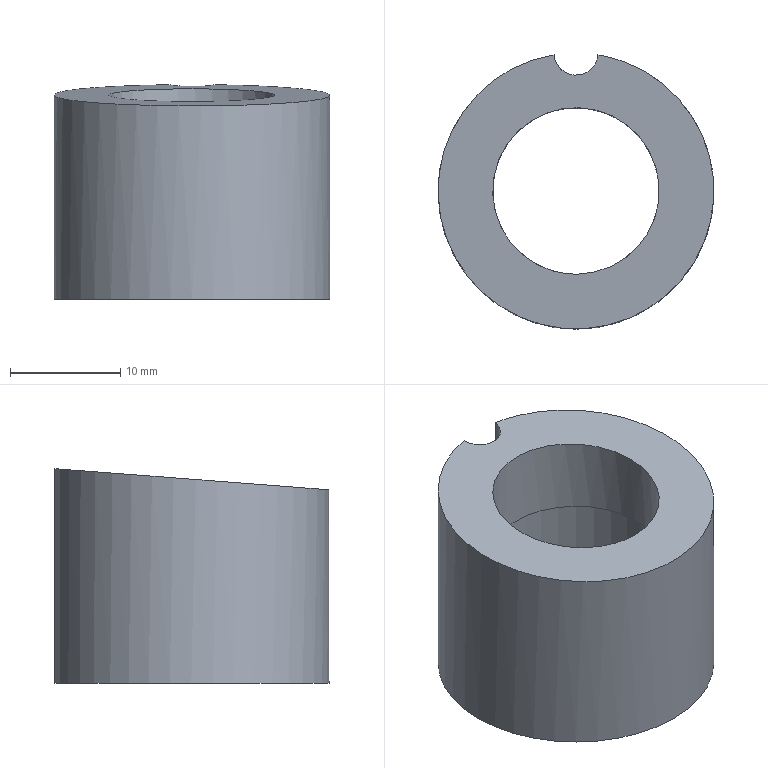Part | NX | features EKSD 25-20-15.10 2 | 1 solid | 7 faces | box 25 x 24.84 x 19.446 mm | volume 5201 mm3 | cylinder 4 | plane 3 | commonest cylinder face diameters 4 x1 15.1 x1 16.6 x1 25 x1
STEP:
#1=CARTESIAN_POINT('',(323.266,-25.835,-35.5));
#2=VERTEX_POINT('',#1);
#3=CARTESIAN_POINT('',(327.253,-25.835,-35.5));
#4=VERTEX_POINT('',#3);
#5=CARTESIAN_POINT('',(325.26,-25.675,-35.5));
#6=DIRECTION('',(0.,0.,1.));
#7=DIRECTION('',(1.,0.,0.));
#8=AXIS2_PLACEMENT_3D('',#5,#6,#7);
#9=CIRCLE('',#8,2.);
#10=EDGE_CURVE('',#2,#4,#9,.T.);
#11=ORIENTED_EDGE('',*,*,#10,.T.);
#12=CARTESIAN_POINT('',(325.26,-38.175,-35.5));
#13=DIRECTION('',(0.,0.,1.));
#14=DIRECTION('',(1.,0.,0.));
#15=AXIS2_PLACEMENT_3D('',#12,#13,#14);
#16=CIRCLE('',#15,12.5);
#17=EDGE_CURVE('',#2,#4,#16,.T.);
#18=ORIENTED_EDGE('',*,*,#17,.F.);
#19=EDGE_LOOP('',(#11,#18));
#20=FACE_BOUND('',#19,.T.);
#21=CARTESIAN_POINT('',(316.96,-38.175,-35.5));
#22=VERTEX_POINT('',#21);
#23=CARTESIAN_POINT('',(325.26,-38.175,-35.5));
#24=DIRECTION('',(0.,0.,-1.));
#25=DIRECTION('',(-1.,0.,0.));
#26=AXIS2_PLACEMENT_3D('',#23,#24,#25);
#27=CIRCLE('',#26,8.3);
#28=EDGE_CURVE('',#22,#22,#27,.T.);
#29=ORIENTED_EDGE('',*,*,#28,.F.);
#30=EDGE_LOOP('',(#29));
#31=FACE_BOUND('',#30,.T.);
#32=CARTESIAN_POINT('',(325.26,-38.175,-35.5));
#33=DIRECTION('',(0.,0.,-1.));
#34=DIRECTION('',(-1.,0.,0.));
#35=AXIS2_PLACEMENT_3D('',#32,#33,#34);
#36=PLANE('',#35);
#37=ADVANCED_FACE('',(#20,#31),#36,.T.);
#38=CARTESIAN_POINT('',(327.253,-25.835,-16.057));
#39=VERTEX_POINT('',#38);
#40=CARTESIAN_POINT('',(323.266,-25.835,-16.054));
#41=VERTEX_POINT('',#40);
#42=CARTESIAN_POINT('',(325.26,-25.675,-16.043));
#43=DIRECTION('',(0.0007587,-0.07675,0.9971));
#44=DIRECTION('',(0.009856,-0.997,-0.07675));
#45=AXIS2_PLACEMENT_3D('',#42,#43,#44);
#46=ELLIPSE('',#45,2.006,2.);
#47=EDGE_CURVE('',#39,#41,#46,.F.);
#48=ORIENTED_EDGE('',*,*,#47,.T.);
#49=CARTESIAN_POINT('',(325.26,-38.175,-17.006));
#50=DIRECTION('',(0.0007587,-0.07675,0.9971));
#51=DIRECTION('',(0.009856,-0.997,-0.07675));
#52=AXIS2_PLACEMENT_3D('',#49,#50,#51);
#53=ELLIPSE('',#52,12.537,12.5);
#54=EDGE_CURVE('',#39,#41,#53,.F.);
#55=ORIENTED_EDGE('',*,*,#54,.F.);
#56=EDGE_LOOP('',(#48,#55));
#57=FACE_BOUND('',#56,.T.);
#58=CARTESIAN_POINT('',(325.334,-45.725,-17.587));
#59=VERTEX_POINT('',#58);
#60=CARTESIAN_POINT('',(325.26,-38.175,-17.006));
#61=DIRECTION('',(0.0007587,-0.07675,0.9971));
#62=DIRECTION('',(0.009856,-0.997,-0.07675));
#63=AXIS2_PLACEMENT_3D('',#60,#61,#62);
#64=ELLIPSE('',#63,7.572,7.55);
#65=EDGE_CURVE('',#59,#59,#64,.T.);
#66=ORIENTED_EDGE('',*,*,#65,.F.);
#67=EDGE_LOOP('',(#66));
#68=FACE_BOUND('',#67,.T.);
#69=CARTESIAN_POINT('',(464.929,116.723,-5.189));
#70=DIRECTION('',(0.0007587,-0.07675,0.9971));
#71=DIRECTION('',(-1.,0.004401,0.0011));
#72=AXIS2_PLACEMENT_3D('',#69,#70,#71);
#73=PLANE('',#72);
#74=ADVANCED_FACE('',(#57,#68),#73,.T.);
#75=CARTESIAN_POINT('',(327.253,-25.835,-25.5));
#76=DIRECTION('',(0.,0.,-1.));
#77=VECTOR('',#76,1000.);
#78=LINE('',#75,#77);
#79=EDGE_CURVE('',#39,#4,#78,.T.);
#80=ORIENTED_EDGE('',*,*,#79,.F.);
#81=ORIENTED_EDGE('',*,*,#54,.T.);
#82=CARTESIAN_POINT('',(323.266,-25.835,-25.5));
#83=DIRECTION('',(0.,0.,-1.));
#84=VECTOR('',#83,1000.);
#85=LINE('',#82,#84);
#86=EDGE_CURVE('',#2,#41,#85,.F.);
#87=ORIENTED_EDGE('',*,*,#86,.F.);
#88=ORIENTED_EDGE('',*,*,#17,.T.);
#89=EDGE_LOOP('',(#80,#81,#87,#88));
#90=FACE_BOUND('',#89,.T.);
#91=CARTESIAN_POINT('',(325.26,-38.175,-15.5));
#92=DIRECTION('',(0.,0.,-1.));
#93=DIRECTION('',(-1.,0.,0.));
#94=AXIS2_PLACEMENT_3D('',#91,#92,#93);
#95=CYLINDRICAL_SURFACE('',#94,12.5);
#96=ADVANCED_FACE('',(#90),#95,.T.);
#97=CARTESIAN_POINT('',(332.81,-38.175,-23.5));
#98=VERTEX_POINT('',#97);
#99=CARTESIAN_POINT('',(325.26,-38.175,-23.5));
#100=DIRECTION('',(0.,0.,1.));
#101=DIRECTION('',(1.,0.,0.));
#102=AXIS2_PLACEMENT_3D('',#99,#100,#101);
#103=CIRCLE('',#102,7.55);
#104=EDGE_CURVE('',#98,#98,#103,.F.);
#105=ORIENTED_EDGE('',*,*,#104,.T.);
#106=EDGE_LOOP('',(#105));
#107=FACE_BOUND('',#106,.T.);
#108=ORIENTED_EDGE('',*,*,#65,.T.);
#109=EDGE_LOOP('',(#108));
#110=FACE_BOUND('',#109,.T.);
#111=CARTESIAN_POINT('',(325.26,-38.175,-14.5));
#112=DIRECTION('',(0.,0.,-1.));
#113=DIRECTION('',(-1.,0.,0.));
#114=AXIS2_PLACEMENT_3D('',#111,#112,#113);
#115=CYLINDRICAL_SURFACE('',#114,7.55);
#116=ADVANCED_FACE('',(#107,#110),#115,.F.);
#117=CARTESIAN_POINT('',(316.96,-38.175,-23.5));
#118=VERTEX_POINT('',#117);
#119=CARTESIAN_POINT('',(325.26,-38.175,-23.5));
#120=DIRECTION('',(0.,0.,-1.));
#121=DIRECTION('',(-1.,0.,0.));
#122=AXIS2_PLACEMENT_3D('',#119,#120,#121);
#123=CIRCLE('',#122,8.3);
#124=EDGE_CURVE('',#118,#118,#123,.T.);
#125=ORIENTED_EDGE('',*,*,#124,.T.);
#126=EDGE_LOOP('',(#125));
#127=FACE_BOUND('',#126,.T.);
#128=ORIENTED_EDGE('',*,*,#104,.F.);
#129=EDGE_LOOP('',(#128));
#130=FACE_BOUND('',#129,.T.);
#131=CARTESIAN_POINT('',(325.26,-38.175,-23.5));
#132=DIRECTION('',(0.,0.,1.));
#133=DIRECTION('',(1.,0.,0.));
#134=AXIS2_PLACEMENT_3D('',#131,#132,#133);
#135=PLANE('',#134);
#136=ADVANCED_FACE('',(#127,#130),#135,.F.);
#137=ORIENTED_EDGE('',*,*,#28,.T.);
#138=EDGE_LOOP('',(#137));
#139=FACE_BOUND('',#138,.T.);
#140=ORIENTED_EDGE('',*,*,#124,.F.);
#141=EDGE_LOOP('',(#140));
#142=FACE_BOUND('',#141,.T.);
#143=CARTESIAN_POINT('',(325.26,-38.175,-23.5));
#144=DIRECTION('',(0.,0.,-1.));
#145=DIRECTION('',(-1.,0.,0.));
#146=AXIS2_PLACEMENT_3D('',#143,#144,#145);
#147=CYLINDRICAL_SURFACE('',#146,8.3);
#148=ADVANCED_FACE('',(#139,#142),#147,.F.);
#149=ORIENTED_EDGE('',*,*,#79,.T.);
#150=ORIENTED_EDGE('',*,*,#10,.F.);
#151=ORIENTED_EDGE('',*,*,#86,.T.);
#152=ORIENTED_EDGE('',*,*,#47,.F.);
#153=EDGE_LOOP('',(#149,#150,#151,#152));
#154=FACE_BOUND('',#153,.T.);
#155=CARTESIAN_POINT('',(325.26,-25.675,-15.5));
#156=DIRECTION('',(0.,0.,-1.));
#157=DIRECTION('',(-1.,0.,0.));
#158=AXIS2_PLACEMENT_3D('',#155,#156,#157);
#159=CYLINDRICAL_SURFACE('',#158,2.);
#160=ADVANCED_FACE('',(#154),#159,.F.);
#161=CLOSED_SHELL('',(#37,#74,#96,#116,#136,#148,#160));
#162=MANIFOLD_SOLID_BREP('',#161);
#163=(LENGTH_UNIT()NAMED_UNIT(*)SI_UNIT(.MILLI.,.METRE.));
#164=UNCERTAINTY_MEASURE_WITH_UNIT(LENGTH_MEASURE(0.00001),#163,'','');
#165=(NAMED_UNIT(*)PLANE_ANGLE_UNIT()SI_UNIT($,.RADIAN.));
#166=(NAMED_UNIT(*)SI_UNIT($,.STERADIAN.)SOLID_ANGLE_UNIT());
#167=(GEOMETRIC_REPRESENTATION_CONTEXT(3)GLOBAL_UNCERTAINTY_ASSIGNED_CONTEXT((#164))GLOBAL_UNIT_ASSIGNED_CONTEXT((#163,#165,#166))REPRESENTATION_CONTEXT('',''));
#168=ADVANCED_BREP_SHAPE_REPRESENTATION('',(#162),#167);